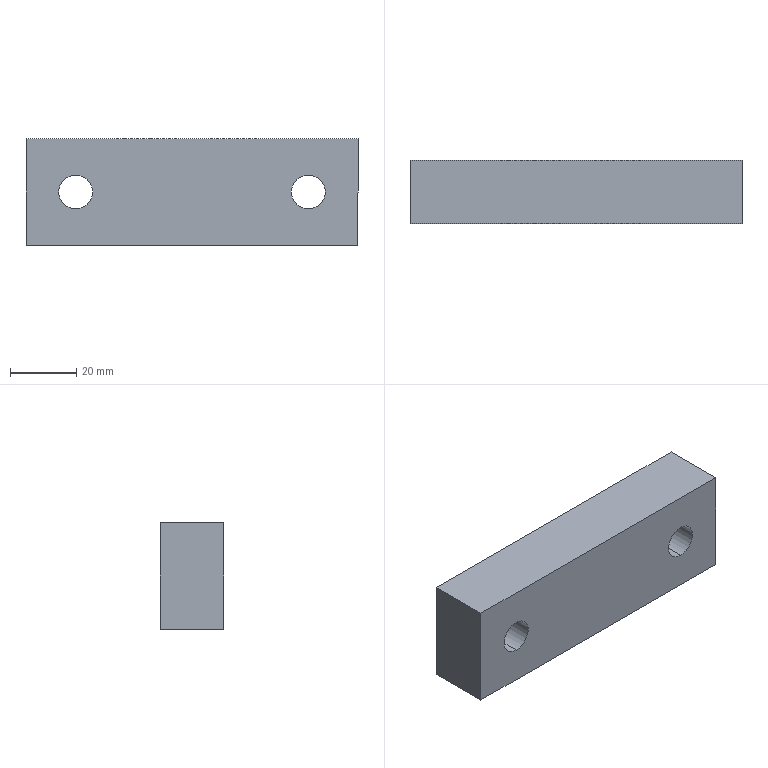Part | SolidWorks | features FlatPattern 1, HoleWzd 1, SMBaseFlange 1, SheetMetal 1 | 1 solid | 10 faces | box 100 x 19 x 32 mm | volume 57695 mm3 | plane 6 | cylinder 4 | commonest cylinder face diameters 10.2 x4
STEP:
#1=CARTESIAN_POINT('',(-35.,-19.,-5.1));
#2=VERTEX_POINT('',#1);
#3=CARTESIAN_POINT('',(-35.,-19.,5.1));
#4=VERTEX_POINT('',#3);
#5=CARTESIAN_POINT('',(-35.,-19.,0.));
#6=DIRECTION('',(0.,1.,0.));
#7=DIRECTION('',(0.,0.,1.));
#8=AXIS2_PLACEMENT_3D('',#5,#6,#7);
#9=CIRCLE('',#8,5.1);
#10=EDGE_CURVE('',#2,#4,#9,.T.);
#11=ORIENTED_EDGE('',*,*,#10,.F.);
#12=CARTESIAN_POINT('',(-35.,0.,-5.1));
#13=VERTEX_POINT('',#12);
#14=CARTESIAN_POINT('',(-35.,0.,-5.1));
#15=DIRECTION('',(0.,1.,0.));
#16=VECTOR('',#15,1000.);
#17=LINE('',#14,#16);
#18=EDGE_CURVE('',#2,#13,#17,.T.);
#19=ORIENTED_EDGE('',*,*,#18,.T.);
#20=CARTESIAN_POINT('',(-35.,0.,5.1));
#21=VERTEX_POINT('',#20);
#22=CARTESIAN_POINT('',(-35.,0.,0.));
#23=DIRECTION('',(0.,1.,0.));
#24=DIRECTION('',(0.,0.,1.));
#25=AXIS2_PLACEMENT_3D('',#22,#23,#24);
#26=CIRCLE('',#25,5.1);
#27=EDGE_CURVE('',#13,#21,#26,.T.);
#28=ORIENTED_EDGE('',*,*,#27,.T.);
#29=CARTESIAN_POINT('',(-35.,0.,5.1));
#30=DIRECTION('',(0.,1.,0.));
#31=VECTOR('',#30,1000.);
#32=LINE('',#29,#31);
#33=EDGE_CURVE('',#4,#21,#32,.T.);
#34=ORIENTED_EDGE('',*,*,#33,.F.);
#35=EDGE_LOOP('',(#11,#19,#28,#34));
#36=FACE_OUTER_BOUND('',#35,.T.);
#37=CARTESIAN_POINT('',(-35.,0.,0.));
#38=DIRECTION('',(0.,1.,0.));
#39=DIRECTION('',(0.,0.,1.));
#40=AXIS2_PLACEMENT_3D('',#37,#38,#39);
#41=CYLINDRICAL_SURFACE('',#40,5.1);
#42=ADVANCED_FACE('',(#36),#41,.F.);
#43=CARTESIAN_POINT('',(35.,-19.,-5.1));
#44=VERTEX_POINT('',#43);
#45=CARTESIAN_POINT('',(35.,-19.,5.1));
#46=VERTEX_POINT('',#45);
#47=CARTESIAN_POINT('',(35.,-19.,0.));
#48=DIRECTION('',(0.,1.,0.));
#49=DIRECTION('',(0.,0.,1.));
#50=AXIS2_PLACEMENT_3D('',#47,#48,#49);
#51=CIRCLE('',#50,5.1);
#52=EDGE_CURVE('',#44,#46,#51,.T.);
#53=ORIENTED_EDGE('',*,*,#52,.F.);
#54=CARTESIAN_POINT('',(35.,0.,-5.1));
#55=VERTEX_POINT('',#54);
#56=CARTESIAN_POINT('',(35.,0.,-5.1));
#57=DIRECTION('',(0.,1.,0.));
#58=VECTOR('',#57,1000.);
#59=LINE('',#56,#58);
#60=EDGE_CURVE('',#44,#55,#59,.T.);
#61=ORIENTED_EDGE('',*,*,#60,.T.);
#62=CARTESIAN_POINT('',(35.,0.,5.1));
#63=VERTEX_POINT('',#62);
#64=CARTESIAN_POINT('',(35.,0.,0.));
#65=DIRECTION('',(0.,1.,0.));
#66=DIRECTION('',(0.,0.,1.));
#67=AXIS2_PLACEMENT_3D('',#64,#65,#66);
#68=CIRCLE('',#67,5.1);
#69=EDGE_CURVE('',#55,#63,#68,.T.);
#70=ORIENTED_EDGE('',*,*,#69,.T.);
#71=CARTESIAN_POINT('',(35.,0.,5.1));
#72=DIRECTION('',(0.,1.,0.));
#73=VECTOR('',#72,1000.);
#74=LINE('',#71,#73);
#75=EDGE_CURVE('',#46,#63,#74,.T.);
#76=ORIENTED_EDGE('',*,*,#75,.F.);
#77=EDGE_LOOP('',(#53,#61,#70,#76));
#78=FACE_OUTER_BOUND('',#77,.T.);
#79=CARTESIAN_POINT('',(35.,0.,0.));
#80=DIRECTION('',(0.,1.,0.));
#81=DIRECTION('',(0.,0.,1.));
#82=AXIS2_PLACEMENT_3D('',#79,#80,#81);
#83=CYLINDRICAL_SURFACE('',#82,5.1);
#84=ADVANCED_FACE('',(#78),#83,.F.);
#85=CARTESIAN_POINT('',(50.,0.,16.));
#86=VERTEX_POINT('',#85);
#87=CARTESIAN_POINT('',(50.,0.,-16.));
#88=VERTEX_POINT('',#87);
#89=CARTESIAN_POINT('',(50.,0.,-16.));
#90=DIRECTION('',(0.,0.,-1.));
#91=VECTOR('',#90,1000.);
#92=LINE('',#89,#91);
#93=EDGE_CURVE('',#86,#88,#92,.T.);
#94=ORIENTED_EDGE('',*,*,#93,.F.);
#95=CARTESIAN_POINT('',(50.,-19.,16.));
#96=VERTEX_POINT('',#95);
#97=CARTESIAN_POINT('',(50.,-19.,16.));
#98=DIRECTION('',(0.,1.,0.));
#99=VECTOR('',#98,1000.);
#100=LINE('',#97,#99);
#101=EDGE_CURVE('',#96,#86,#100,.T.);
#102=ORIENTED_EDGE('',*,*,#101,.F.);
#103=CARTESIAN_POINT('',(50.,-19.,-16.));
#104=VERTEX_POINT('',#103);
#105=CARTESIAN_POINT('',(50.,-19.,-16.));
#106=DIRECTION('',(0.,0.,-1.));
#107=VECTOR('',#106,1000.);
#108=LINE('',#105,#107);
#109=EDGE_CURVE('',#96,#104,#108,.T.);
#110=ORIENTED_EDGE('',*,*,#109,.T.);
#111=CARTESIAN_POINT('',(50.,-19.,-16.));
#112=DIRECTION('',(0.,1.,0.));
#113=VECTOR('',#112,1000.);
#114=LINE('',#111,#113);
#115=EDGE_CURVE('',#104,#88,#114,.T.);
#116=ORIENTED_EDGE('',*,*,#115,.T.);
#117=EDGE_LOOP('',(#94,#102,#110,#116));
#118=FACE_OUTER_BOUND('',#117,.T.);
#119=CARTESIAN_POINT('',(50.,-19.,-16.));
#120=DIRECTION('',(1.,0.,0.));
#121=DIRECTION('',(0.,0.,-1.));
#122=AXIS2_PLACEMENT_3D('',#119,#120,#121);
#123=PLANE('',#122);
#124=ADVANCED_FACE('',(#118),#123,.T.);
#125=CARTESIAN_POINT('',(-50.,0.,16.));
#126=VERTEX_POINT('',#125);
#127=CARTESIAN_POINT('',(-50.,0.,16.));
#128=DIRECTION('',(1.,0.,0.));
#129=VECTOR('',#128,1000.);
#130=LINE('',#127,#129);
#131=EDGE_CURVE('',#126,#86,#130,.T.);
#132=ORIENTED_EDGE('',*,*,#131,.F.);
#133=CARTESIAN_POINT('',(-50.,-19.,16.));
#134=VERTEX_POINT('',#133);
#135=CARTESIAN_POINT('',(-50.,-19.,16.));
#136=DIRECTION('',(0.,1.,0.));
#137=VECTOR('',#136,1000.);
#138=LINE('',#135,#137);
#139=EDGE_CURVE('',#134,#126,#138,.T.);
#140=ORIENTED_EDGE('',*,*,#139,.F.);
#141=CARTESIAN_POINT('',(-50.,-19.,16.));
#142=DIRECTION('',(1.,0.,0.));
#143=VECTOR('',#142,1000.);
#144=LINE('',#141,#143);
#145=EDGE_CURVE('',#134,#96,#144,.T.);
#146=ORIENTED_EDGE('',*,*,#145,.T.);
#147=ORIENTED_EDGE('',*,*,#101,.T.);
#148=EDGE_LOOP('',(#132,#140,#146,#147));
#149=FACE_OUTER_BOUND('',#148,.T.);
#150=CARTESIAN_POINT('',(-50.,-19.,16.));
#151=DIRECTION('',(0.,0.,1.));
#152=DIRECTION('',(1.,0.,0.));
#153=AXIS2_PLACEMENT_3D('',#150,#151,#152);
#154=PLANE('',#153);
#155=ADVANCED_FACE('',(#149),#154,.T.);
#156=CARTESIAN_POINT('',(-50.,0.,-16.));
#157=VERTEX_POINT('',#156);
#158=CARTESIAN_POINT('',(-50.,0.,-16.));
#159=DIRECTION('',(0.,0.,1.));
#160=VECTOR('',#159,1000.);
#161=LINE('',#158,#160);
#162=EDGE_CURVE('',#157,#126,#161,.T.);
#163=ORIENTED_EDGE('',*,*,#162,.F.);
#164=CARTESIAN_POINT('',(-50.,-19.,-16.));
#165=VERTEX_POINT('',#164);
#166=CARTESIAN_POINT('',(-50.,-19.,-16.));
#167=DIRECTION('',(0.,1.,0.));
#168=VECTOR('',#167,1000.);
#169=LINE('',#166,#168);
#170=EDGE_CURVE('',#165,#157,#169,.T.);
#171=ORIENTED_EDGE('',*,*,#170,.F.);
#172=CARTESIAN_POINT('',(-50.,-19.,-16.));
#173=DIRECTION('',(0.,0.,1.));
#174=VECTOR('',#173,1000.);
#175=LINE('',#172,#174);
#176=EDGE_CURVE('',#165,#134,#175,.T.);
#177=ORIENTED_EDGE('',*,*,#176,.T.);
#178=ORIENTED_EDGE('',*,*,#139,.T.);
#179=EDGE_LOOP('',(#163,#171,#177,#178));
#180=FACE_OUTER_BOUND('',#179,.T.);
#181=CARTESIAN_POINT('',(-50.,-19.,-16.));
#182=DIRECTION('',(-1.,0.,0.));
#183=DIRECTION('',(0.,0.,1.));
#184=AXIS2_PLACEMENT_3D('',#181,#182,#183);
#185=PLANE('',#184);
#186=ADVANCED_FACE('',(#180),#185,.T.);
#187=CARTESIAN_POINT('',(-50.,0.,-16.));
#188=DIRECTION('',(-1.,0.,0.));
#189=VECTOR('',#188,1000.);
#190=LINE('',#187,#189);
#191=EDGE_CURVE('',#88,#157,#190,.T.);
#192=ORIENTED_EDGE('',*,*,#191,.F.);
#193=ORIENTED_EDGE('',*,*,#115,.F.);
#194=CARTESIAN_POINT('',(-50.,-19.,-16.));
#195=DIRECTION('',(-1.,0.,0.));
#196=VECTOR('',#195,1000.);
#197=LINE('',#194,#196);
#198=EDGE_CURVE('',#104,#165,#197,.T.);
#199=ORIENTED_EDGE('',*,*,#198,.T.);
#200=ORIENTED_EDGE('',*,*,#170,.T.);
#201=EDGE_LOOP('',(#192,#193,#199,#200));
#202=FACE_OUTER_BOUND('',#201,.T.);
#203=CARTESIAN_POINT('',(-50.,-19.,-16.));
#204=DIRECTION('',(0.,0.,-1.));
#205=DIRECTION('',(-1.,0.,0.));
#206=AXIS2_PLACEMENT_3D('',#203,#204,#205);
#207=PLANE('',#206);
#208=ADVANCED_FACE('',(#202),#207,.T.);
#209=CARTESIAN_POINT('',(-35.,-19.,0.));
#210=DIRECTION('',(0.,1.,0.));
#211=DIRECTION('',(0.,0.,1.));
#212=AXIS2_PLACEMENT_3D('',#209,#210,#211);
#213=CIRCLE('',#212,5.1);
#214=EDGE_CURVE('',#4,#2,#213,.T.);
#215=ORIENTED_EDGE('',*,*,#214,.T.);
#216=ORIENTED_EDGE('',*,*,#10,.T.);
#217=EDGE_LOOP('',(#215,#216));
#218=FACE_BOUND('',#217,.T.);
#219=CARTESIAN_POINT('',(35.,-19.,0.));
#220=DIRECTION('',(0.,1.,0.));
#221=DIRECTION('',(0.,0.,1.));
#222=AXIS2_PLACEMENT_3D('',#219,#220,#221);
#223=CIRCLE('',#222,5.1);
#224=EDGE_CURVE('',#46,#44,#223,.T.);
#225=ORIENTED_EDGE('',*,*,#224,.T.);
#226=ORIENTED_EDGE('',*,*,#52,.T.);
#227=EDGE_LOOP('',(#225,#226));
#228=FACE_BOUND('',#227,.T.);
#229=ORIENTED_EDGE('',*,*,#109,.F.);
#230=ORIENTED_EDGE('',*,*,#145,.F.);
#231=ORIENTED_EDGE('',*,*,#176,.F.);
#232=ORIENTED_EDGE('',*,*,#198,.F.);
#233=EDGE_LOOP('',(#229,#230,#231,#232));
#234=FACE_OUTER_BOUND('',#233,.T.);
#235=CARTESIAN_POINT('',(0.,-19.,0.));
#236=DIRECTION('',(0.,1.,0.));
#237=DIRECTION('',(0.,0.,1.));
#238=AXIS2_PLACEMENT_3D('',#235,#236,#237);
#239=PLANE('',#238);
#240=ADVANCED_FACE('',(#218,#228,#234),#239,.F.);
#241=CARTESIAN_POINT('',(-35.,0.,0.));
#242=DIRECTION('',(0.,1.,0.));
#243=DIRECTION('',(0.,0.,1.));
#244=AXIS2_PLACEMENT_3D('',#241,#242,#243);
#245=CIRCLE('',#244,5.1);
#246=EDGE_CURVE('',#21,#13,#245,.T.);
#247=ORIENTED_EDGE('',*,*,#246,.F.);
#248=ORIENTED_EDGE('',*,*,#27,.F.);
#249=EDGE_LOOP('',(#247,#248));
#250=FACE_BOUND('',#249,.T.);
#251=CARTESIAN_POINT('',(35.,0.,0.));
#252=DIRECTION('',(0.,1.,0.));
#253=DIRECTION('',(0.,0.,1.));
#254=AXIS2_PLACEMENT_3D('',#251,#252,#253);
#255=CIRCLE('',#254,5.1);
#256=EDGE_CURVE('',#63,#55,#255,.T.);
#257=ORIENTED_EDGE('',*,*,#256,.F.);
#258=ORIENTED_EDGE('',*,*,#69,.F.);
#259=EDGE_LOOP('',(#257,#258));
#260=FACE_BOUND('',#259,.T.);
#261=ORIENTED_EDGE('',*,*,#93,.T.);
#262=ORIENTED_EDGE('',*,*,#191,.T.);
#263=ORIENTED_EDGE('',*,*,#162,.T.);
#264=ORIENTED_EDGE('',*,*,#131,.T.);
#265=EDGE_LOOP('',(#261,#262,#263,#264));
#266=FACE_OUTER_BOUND('',#265,.T.);
#267=CARTESIAN_POINT('',(0.,0.,0.));
#268=DIRECTION('',(0.,1.,0.));
#269=DIRECTION('',(0.,0.,1.));
#270=AXIS2_PLACEMENT_3D('',#267,#268,#269);
#271=PLANE('',#270);
#272=ADVANCED_FACE('',(#250,#260,#266),#271,.T.);
#273=ORIENTED_EDGE('',*,*,#60,.F.);
#274=ORIENTED_EDGE('',*,*,#224,.F.);
#275=ORIENTED_EDGE('',*,*,#75,.T.);
#276=ORIENTED_EDGE('',*,*,#256,.T.);
#277=EDGE_LOOP('',(#273,#274,#275,#276));
#278=FACE_OUTER_BOUND('',#277,.T.);
#279=CARTESIAN_POINT('',(35.,0.,0.));
#280=DIRECTION('',(0.,1.,0.));
#281=DIRECTION('',(0.,0.,1.));
#282=AXIS2_PLACEMENT_3D('',#279,#280,#281);
#283=CYLINDRICAL_SURFACE('',#282,5.1);
#284=ADVANCED_FACE('',(#278),#283,.F.);
#285=ORIENTED_EDGE('',*,*,#18,.F.);
#286=ORIENTED_EDGE('',*,*,#214,.F.);
#287=ORIENTED_EDGE('',*,*,#33,.T.);
#288=ORIENTED_EDGE('',*,*,#246,.T.);
#289=EDGE_LOOP('',(#285,#286,#287,#288));
#290=FACE_OUTER_BOUND('',#289,.T.);
#291=CARTESIAN_POINT('',(-35.,0.,0.));
#292=DIRECTION('',(0.,1.,0.));
#293=DIRECTION('',(0.,0.,1.));
#294=AXIS2_PLACEMENT_3D('',#291,#292,#293);
#295=CYLINDRICAL_SURFACE('',#294,5.1);
#296=ADVANCED_FACE('',(#290),#295,.F.);
#297=CLOSED_SHELL('',(#42,#84,#124,#155,#186,#208,#240,#272,#284,#296));
#298=MANIFOLD_SOLID_BREP('',#297);
#299=CARTESIAN_POINT('',(0.,0.,0.));
#300=DIRECTION('',(0.,0.,1.));
#301=DIRECTION('',(1.,0.,0.));
#302=AXIS2_PLACEMENT_3D('',#299,#300,#301);
#303=(LENGTH_UNIT()NAMED_UNIT(*)SI_UNIT(.MILLI.,.METRE.));
#304=UNCERTAINTY_MEASURE_WITH_UNIT(LENGTH_MEASURE(0.00001),#303,'','');
#305=(NAMED_UNIT(*)PLANE_ANGLE_UNIT()SI_UNIT($,.RADIAN.));
#306=(NAMED_UNIT(*)SI_UNIT($,.STERADIAN.)SOLID_ANGLE_UNIT());
#307=(GEOMETRIC_REPRESENTATION_CONTEXT(3)GLOBAL_UNCERTAINTY_ASSIGNED_CONTEXT((#304))GLOBAL_UNIT_ASSIGNED_CONTEXT((#303,#305,#306))REPRESENTATION_CONTEXT('',''));
#308=ADVANCED_BREP_SHAPE_REPRESENTATION('',(#298,#302),#307);